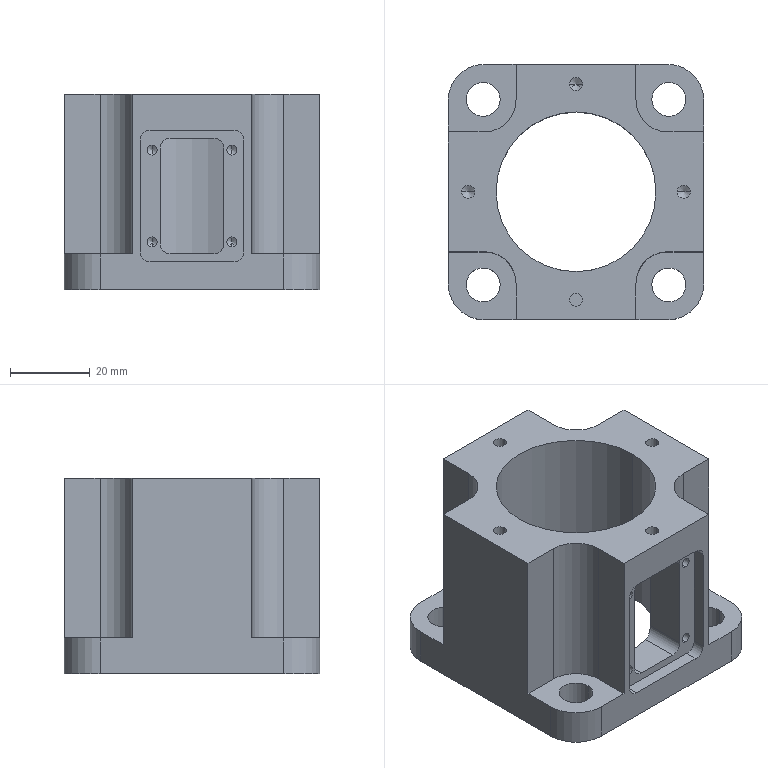Part | SolidWorks | features BaseBody 1 | 1 solid | 86 faces | box 64 x 64 x 49 mm | volume 81179 mm3 | cylinder 44 | plane 28 | cone 14 | commonest cylinder face diameters 2.5 x8 3.3 x8 5 x8 8.5 x8 16 x4 18 x4